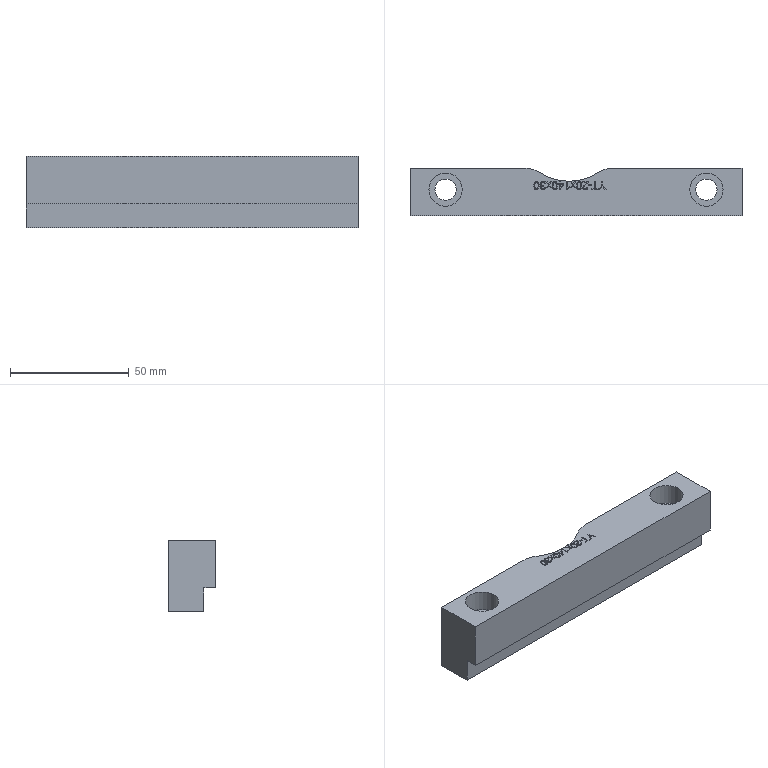Part | STEP file | lll_id358_x_t | 1 solid | 171 faces | box 140 x 20 x 30 mm | volume 68147 mm3 | plane 100 | other 64 | cylinder 7 | commonest cylinder face diameters 9 x2 14 x2 20 x2 45 x1